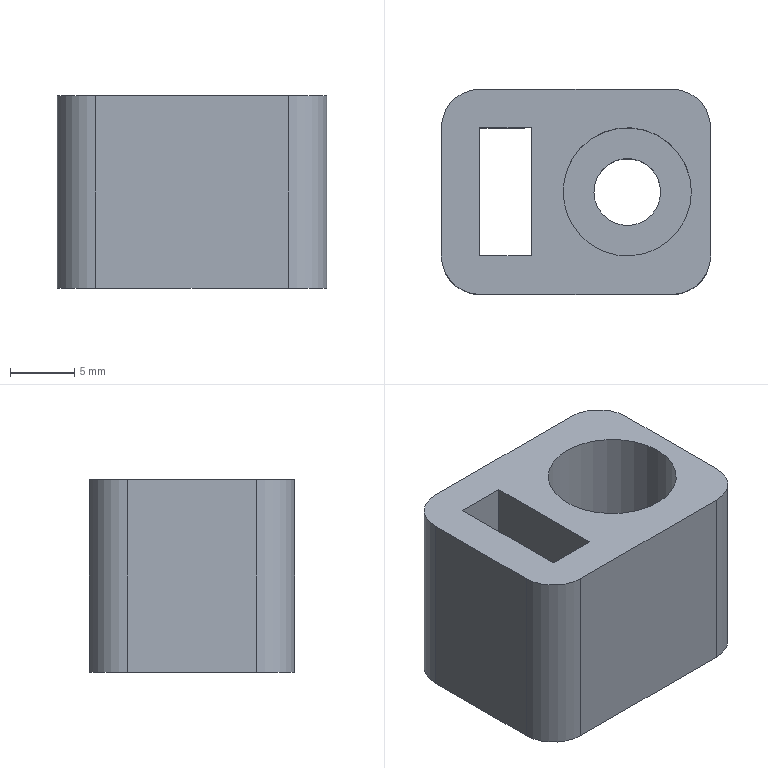Part | NX | features DIE-17 2 | 1 solid | 25 faces | box 21 x 16 x 15 mm | volume 3498 mm3 | plane 15 | cylinder 10 | commonest cylinder face diameters 2 x4 6 x4 5.206 x1 10 x1
STEP:
#1=CARTESIAN_POINT('',(2422.893,-834.621,858.716));
#2=VERTEX_POINT('',#1);
#3=CARTESIAN_POINT('',(2422.893,-834.621,846.716));
#4=VERTEX_POINT('',#3);
#5=CARTESIAN_POINT('',(2422.893,-834.621,858.516));
#6=DIRECTION('',(0.,0.,-1.));
#7=VECTOR('',#6,1000.);
#8=LINE('',#5,#7);
#9=EDGE_CURVE('',#2,#4,#8,.T.);
#10=ORIENTED_EDGE('',*,*,#9,.T.);
#11=CARTESIAN_POINT('',(2422.893,-844.621,846.716));
#12=VERTEX_POINT('',#11);
#13=CARTESIAN_POINT('',(2422.893,-833.746,846.716));
#14=DIRECTION('',(0.,1.,0.));
#15=VECTOR('',#14,1000.);
#16=LINE('',#13,#15);
#17=EDGE_CURVE('',#12,#4,#16,.T.);
#18=ORIENTED_EDGE('',*,*,#17,.F.);
#19=CARTESIAN_POINT('',(2422.893,-844.621,858.716));
#20=VERTEX_POINT('',#19);
#21=CARTESIAN_POINT('',(2422.893,-844.621,858.516));
#22=DIRECTION('',(0.,0.,-1.));
#23=VECTOR('',#22,1000.);
#24=LINE('',#21,#23);
#25=EDGE_CURVE('',#20,#12,#24,.T.);
#26=ORIENTED_EDGE('',*,*,#25,.F.);
#27=CARTESIAN_POINT('',(2422.893,-839.621,858.716));
#28=DIRECTION('',(0.,-1.,0.));
#29=VECTOR('',#28,1000.);
#30=LINE('',#27,#29);
#31=EDGE_CURVE('',#20,#2,#30,.F.);
#32=ORIENTED_EDGE('',*,*,#31,.T.);
#33=EDGE_LOOP('',(#10,#18,#26,#32));
#34=FACE_BOUND('',#33,.T.);
#35=CARTESIAN_POINT('',(2422.893,-837.246,858.516));
#36=DIRECTION('',(-1.,0.,0.));
#37=DIRECTION('',(0.,0.,1.));
#38=AXIS2_PLACEMENT_3D('',#35,#36,#37);
#39=PLANE('',#38);
#40=ADVANCED_FACE('',(#34),#39,.T.);
#41=CARTESIAN_POINT('',(2418.893,-834.621,858.716));
#42=VERTEX_POINT('',#41);
#43=CARTESIAN_POINT('',(2420.893,-834.621,858.716));
#44=DIRECTION('',(1.,0.,0.));
#45=VECTOR('',#44,1000.);
#46=LINE('',#43,#45);
#47=EDGE_CURVE('',#2,#42,#46,.F.);
#48=ORIENTED_EDGE('',*,*,#47,.F.);
#49=ORIENTED_EDGE('',*,*,#31,.F.);
#50=CARTESIAN_POINT('',(2418.893,-844.621,858.716));
#51=VERTEX_POINT('',#50);
#52=CARTESIAN_POINT('',(2420.893,-844.621,858.716));
#53=DIRECTION('',(1.,0.,0.));
#54=VECTOR('',#53,1000.);
#55=LINE('',#52,#54);
#56=EDGE_CURVE('',#20,#51,#55,.F.);
#57=ORIENTED_EDGE('',*,*,#56,.T.);
#58=CARTESIAN_POINT('',(2418.893,-837.871,858.716));
#59=DIRECTION('',(0.,-1.,0.));
#60=VECTOR('',#59,1000.);
#61=LINE('',#58,#60);
#62=EDGE_CURVE('',#42,#51,#61,.T.);
#63=ORIENTED_EDGE('',*,*,#62,.F.);
#64=EDGE_LOOP('',(#48,#49,#57,#63));
#65=FACE_BOUND('',#64,.T.);
#66=CARTESIAN_POINT('',(2415.893,-844.621,858.716));
#67=VERTEX_POINT('',#66);
#68=CARTESIAN_POINT('',(2418.893,-847.621,858.716));
#69=VERTEX_POINT('',#68);
#70=CARTESIAN_POINT('',(2418.893,-844.621,858.716));
#71=DIRECTION('',(0.,0.,1.));
#72=DIRECTION('',(1.,0.,0.));
#73=AXIS2_PLACEMENT_3D('',#70,#71,#72);
#74=CIRCLE('',#73,3.);
#75=EDGE_CURVE('',#67,#69,#74,.T.);
#76=ORIENTED_EDGE('',*,*,#75,.T.);
#77=CARTESIAN_POINT('',(2433.893,-847.621,858.716));
#78=VERTEX_POINT('',#77);
#79=CARTESIAN_POINT('',(2421.393,-847.621,858.716));
#80=DIRECTION('',(-1.,0.,0.));
#81=VECTOR('',#80,1000.);
#82=LINE('',#79,#81);
#83=EDGE_CURVE('',#78,#69,#82,.T.);
#84=ORIENTED_EDGE('',*,*,#83,.F.);
#85=CARTESIAN_POINT('',(2436.893,-844.621,858.716));
#86=VERTEX_POINT('',#85);
#87=CARTESIAN_POINT('',(2433.893,-844.621,858.716));
#88=DIRECTION('',(0.,0.,1.));
#89=DIRECTION('',(1.,0.,0.));
#90=AXIS2_PLACEMENT_3D('',#87,#88,#89);
#91=CIRCLE('',#90,3.);
#92=EDGE_CURVE('',#78,#86,#91,.T.);
#93=ORIENTED_EDGE('',*,*,#92,.T.);
#94=CARTESIAN_POINT('',(2436.893,-834.621,858.716));
#95=VERTEX_POINT('',#94);
#96=CARTESIAN_POINT('',(2436.893,-839.621,858.716));
#97=DIRECTION('',(0.,-1.,0.));
#98=VECTOR('',#97,1000.);
#99=LINE('',#96,#98);
#100=EDGE_CURVE('',#95,#86,#99,.T.);
#101=ORIENTED_EDGE('',*,*,#100,.F.);
#102=CARTESIAN_POINT('',(2433.893,-831.621,858.716));
#103=VERTEX_POINT('',#102);
#104=CARTESIAN_POINT('',(2433.893,-834.621,858.716));
#105=DIRECTION('',(0.,0.,1.));
#106=DIRECTION('',(1.,0.,0.));
#107=AXIS2_PLACEMENT_3D('',#104,#105,#106);
#108=CIRCLE('',#107,3.);
#109=EDGE_CURVE('',#95,#103,#108,.T.);
#110=ORIENTED_EDGE('',*,*,#109,.T.);
#111=CARTESIAN_POINT('',(2418.893,-831.621,858.716));
#112=VERTEX_POINT('',#111);
#113=CARTESIAN_POINT('',(2421.393,-831.621,858.716));
#114=DIRECTION('',(1.,0.,0.));
#115=VECTOR('',#114,1000.);
#116=LINE('',#113,#115);
#117=EDGE_CURVE('',#112,#103,#116,.T.);
#118=ORIENTED_EDGE('',*,*,#117,.F.);
#119=CARTESIAN_POINT('',(2415.893,-834.621,858.716));
#120=VERTEX_POINT('',#119);
#121=CARTESIAN_POINT('',(2418.893,-834.621,858.716));
#122=DIRECTION('',(0.,0.,1.));
#123=DIRECTION('',(1.,0.,0.));
#124=AXIS2_PLACEMENT_3D('',#121,#122,#123);
#125=CIRCLE('',#124,3.);
#126=EDGE_CURVE('',#112,#120,#125,.T.);
#127=ORIENTED_EDGE('',*,*,#126,.T.);
#128=CARTESIAN_POINT('',(2415.893,-839.621,858.716));
#129=DIRECTION('',(0.,1.,0.));
#130=VECTOR('',#129,1000.);
#131=LINE('',#128,#130);
#132=EDGE_CURVE('',#67,#120,#131,.T.);
#133=ORIENTED_EDGE('',*,*,#132,.F.);
#134=EDGE_LOOP('',(#76,#84,#93,#101,#110,#118,#127,#133));
#135=FACE_BOUND('',#134,.T.);
#136=CARTESIAN_POINT('',(2435.393,-839.621,858.716));
#137=VERTEX_POINT('',#136);
#138=CARTESIAN_POINT('',(2430.393,-839.621,858.716));
#139=DIRECTION('',(0.,0.,1.));
#140=DIRECTION('',(1.,0.,0.));
#141=AXIS2_PLACEMENT_3D('',#138,#139,#140);
#142=CIRCLE('',#141,5.);
#143=EDGE_CURVE('',#137,#137,#142,.T.);
#144=ORIENTED_EDGE('',*,*,#143,.F.);
#145=EDGE_LOOP('',(#144));
#146=FACE_BOUND('',#145,.T.);
#147=CARTESIAN_POINT('',(2421.393,-839.621,858.716));
#148=DIRECTION('',(0.,0.,1.));
#149=DIRECTION('',(1.,0.,0.));
#150=AXIS2_PLACEMENT_3D('',#147,#148,#149);
#151=PLANE('',#150);
#152=ADVANCED_FACE('',(#65,#135,#146),#151,.T.);
#153=CARTESIAN_POINT('',(2418.893,-844.621,843.716));
#154=VERTEX_POINT('',#153);
#155=CARTESIAN_POINT('',(2422.393,-844.621,843.716));
#156=VERTEX_POINT('',#155);
#157=CARTESIAN_POINT('',(2422.281,-844.621,843.716));
#158=DIRECTION('',(1.,0.,0.));
#159=VECTOR('',#158,1000.);
#160=LINE('',#157,#159);
#161=EDGE_CURVE('',#154,#156,#160,.T.);
#162=ORIENTED_EDGE('',*,*,#161,.T.);
#163=CARTESIAN_POINT('',(2423.259,-845.121,843.716));
#164=VERTEX_POINT('',#163);
#165=CARTESIAN_POINT('',(2423.259,-844.121,843.716));
#166=DIRECTION('',(0.,0.,-1.));
#167=DIRECTION('',(-1.,0.,0.));
#168=AXIS2_PLACEMENT_3D('',#165,#166,#167);
#169=CIRCLE('',#168,1.);
#170=EDGE_CURVE('',#156,#164,#169,.F.);
#171=ORIENTED_EDGE('',*,*,#170,.T.);
#172=CARTESIAN_POINT('',(2423.393,-845.121,843.716));
#173=VERTEX_POINT('',#172);
#174=CARTESIAN_POINT('',(2421.393,-845.121,843.716));
#175=DIRECTION('',(1.,0.,0.));
#176=VECTOR('',#175,1000.);
#177=LINE('',#174,#176);
#178=EDGE_CURVE('',#164,#173,#177,.T.);
#179=ORIENTED_EDGE('',*,*,#178,.T.);
#180=CARTESIAN_POINT('',(2424.393,-844.121,843.716));
#181=VERTEX_POINT('',#180);
#182=CARTESIAN_POINT('',(2423.393,-844.121,843.716));
#183=DIRECTION('',(0.,0.,-1.));
#184=DIRECTION('',(-1.,0.,0.));
#185=AXIS2_PLACEMENT_3D('',#182,#183,#184);
#186=CIRCLE('',#185,1.);
#187=EDGE_CURVE('',#173,#181,#186,.F.);
#188=ORIENTED_EDGE('',*,*,#187,.T.);
#189=CARTESIAN_POINT('',(2424.393,-835.121,843.716));
#190=VERTEX_POINT('',#189);
#191=CARTESIAN_POINT('',(2424.393,-833.746,843.716));
#192=DIRECTION('',(0.,-1.,0.));
#193=VECTOR('',#192,1000.);
#194=LINE('',#191,#193);
#195=EDGE_CURVE('',#190,#181,#194,.T.);
#196=ORIENTED_EDGE('',*,*,#195,.F.);
#197=CARTESIAN_POINT('',(2423.393,-834.121,843.716));
#198=VERTEX_POINT('',#197);
#199=CARTESIAN_POINT('',(2423.393,-835.121,843.716));
#200=DIRECTION('',(0.,0.,-1.));
#201=DIRECTION('',(-1.,0.,0.));
#202=AXIS2_PLACEMENT_3D('',#199,#200,#201);
#203=CIRCLE('',#202,1.);
#204=EDGE_CURVE('',#190,#198,#203,.F.);
#205=ORIENTED_EDGE('',*,*,#204,.T.);
#206=CARTESIAN_POINT('',(2423.259,-834.121,843.716));
#207=VERTEX_POINT('',#206);
#208=CARTESIAN_POINT('',(2421.393,-834.121,843.716));
#209=DIRECTION('',(-1.,0.,0.));
#210=VECTOR('',#209,1000.);
#211=LINE('',#208,#210);
#212=EDGE_CURVE('',#198,#207,#211,.T.);
#213=ORIENTED_EDGE('',*,*,#212,.T.);
#214=CARTESIAN_POINT('',(2422.393,-834.621,843.716));
#215=VERTEX_POINT('',#214);
#216=CARTESIAN_POINT('',(2423.259,-835.121,843.716));
#217=DIRECTION('',(0.,0.,-1.));
#218=DIRECTION('',(-1.,0.,0.));
#219=AXIS2_PLACEMENT_3D('',#216,#217,#218);
#220=CIRCLE('',#219,1.);
#221=EDGE_CURVE('',#207,#215,#220,.F.);
#222=ORIENTED_EDGE('',*,*,#221,.T.);
#223=CARTESIAN_POINT('',(2418.893,-834.621,843.716));
#224=VERTEX_POINT('',#223);
#225=CARTESIAN_POINT('',(2422.281,-834.621,843.716));
#226=DIRECTION('',(-1.,0.,0.));
#227=VECTOR('',#226,1000.);
#228=LINE('',#225,#227);
#229=EDGE_CURVE('',#215,#224,#228,.T.);
#230=ORIENTED_EDGE('',*,*,#229,.T.);
#231=CARTESIAN_POINT('',(2418.893,-833.746,843.716));
#232=DIRECTION('',(0.,-1.,0.));
#233=VECTOR('',#232,1000.);
#234=LINE('',#231,#233);
#235=EDGE_CURVE('',#224,#154,#234,.T.);
#236=ORIENTED_EDGE('',*,*,#235,.T.);
#237=EDGE_LOOP('',(#162,#171,#179,#188,#196,#205,#213,#222,#230,#236));
#238=FACE_BOUND('',#237,.T.);
#239=CARTESIAN_POINT('',(2427.79,-839.621,843.716));
#240=VERTEX_POINT('',#239);
#241=CARTESIAN_POINT('',(2430.393,-839.621,843.716));
#242=DIRECTION('',(0.,0.,-1.));
#243=DIRECTION('',(-1.,0.,0.));
#244=AXIS2_PLACEMENT_3D('',#241,#242,#243);
#245=CIRCLE('',#244,2.603);
#246=EDGE_CURVE('',#240,#240,#245,.T.);
#247=ORIENTED_EDGE('',*,*,#246,.F.);
#248=EDGE_LOOP('',(#247));
#249=FACE_BOUND('',#248,.T.);
#250=CARTESIAN_POINT('',(2418.893,-847.621,843.716));
#251=VERTEX_POINT('',#250);
#252=CARTESIAN_POINT('',(2433.893,-847.621,843.716));
#253=VERTEX_POINT('',#252);
#254=CARTESIAN_POINT('',(2421.393,-847.621,843.716));
#255=DIRECTION('',(1.,0.,0.));
#256=VECTOR('',#255,1000.);
#257=LINE('',#254,#256);
#258=EDGE_CURVE('',#251,#253,#257,.T.);
#259=ORIENTED_EDGE('',*,*,#258,.F.);
#260=CARTESIAN_POINT('',(2415.893,-844.621,843.716));
#261=VERTEX_POINT('',#260);
#262=CARTESIAN_POINT('',(2418.893,-844.621,843.716));
#263=DIRECTION('',(0.,0.,-1.));
#264=DIRECTION('',(-1.,0.,0.));
#265=AXIS2_PLACEMENT_3D('',#262,#263,#264);
#266=CIRCLE('',#265,3.);
#267=EDGE_CURVE('',#251,#261,#266,.T.);
#268=ORIENTED_EDGE('',*,*,#267,.T.);
#269=CARTESIAN_POINT('',(2415.893,-834.621,843.716));
#270=VERTEX_POINT('',#269);
#271=CARTESIAN_POINT('',(2415.893,-839.621,843.716));
#272=DIRECTION('',(0.,-1.,0.));
#273=VECTOR('',#272,1000.);
#274=LINE('',#271,#273);
#275=EDGE_CURVE('',#270,#261,#274,.T.);
#276=ORIENTED_EDGE('',*,*,#275,.F.);
#277=CARTESIAN_POINT('',(2418.893,-831.621,843.716));
#278=VERTEX_POINT('',#277);
#279=CARTESIAN_POINT('',(2418.893,-834.621,843.716));
#280=DIRECTION('',(0.,0.,-1.));
#281=DIRECTION('',(-1.,0.,0.));
#282=AXIS2_PLACEMENT_3D('',#279,#280,#281);
#283=CIRCLE('',#282,3.);
#284=EDGE_CURVE('',#270,#278,#283,.T.);
#285=ORIENTED_EDGE('',*,*,#284,.T.);
#286=CARTESIAN_POINT('',(2433.893,-831.621,843.716));
#287=VERTEX_POINT('',#286);
#288=CARTESIAN_POINT('',(2421.393,-831.621,843.716));
#289=DIRECTION('',(-1.,0.,0.));
#290=VECTOR('',#289,1000.);
#291=LINE('',#288,#290);
#292=EDGE_CURVE('',#287,#278,#291,.T.);
#293=ORIENTED_EDGE('',*,*,#292,.F.);
#294=CARTESIAN_POINT('',(2436.893,-834.621,843.716));
#295=VERTEX_POINT('',#294);
#296=CARTESIAN_POINT('',(2433.893,-834.621,843.716));
#297=DIRECTION('',(0.,0.,-1.));
#298=DIRECTION('',(-1.,0.,0.));
#299=AXIS2_PLACEMENT_3D('',#296,#297,#298);
#300=CIRCLE('',#299,3.);
#301=EDGE_CURVE('',#287,#295,#300,.T.);
#302=ORIENTED_EDGE('',*,*,#301,.T.);
#303=CARTESIAN_POINT('',(2436.893,-844.621,843.716));
#304=VERTEX_POINT('',#303);
#305=CARTESIAN_POINT('',(2436.893,-839.621,843.716));
#306=DIRECTION('',(0.,1.,0.));
#307=VECTOR('',#306,1000.);
#308=LINE('',#305,#307);
#309=EDGE_CURVE('',#304,#295,#308,.T.);
#310=ORIENTED_EDGE('',*,*,#309,.F.);
#311=CARTESIAN_POINT('',(2433.893,-844.621,843.716));
#312=DIRECTION('',(0.,0.,-1.));
#313=DIRECTION('',(-1.,0.,0.));
#314=AXIS2_PLACEMENT_3D('',#311,#312,#313);
#315=CIRCLE('',#314,3.);
#316=EDGE_CURVE('',#304,#253,#315,.T.);
#317=ORIENTED_EDGE('',*,*,#316,.T.);
#318=EDGE_LOOP('',(#259,#268,#276,#285,#293,#302,#310,#317));
#319=FACE_BOUND('',#318,.T.);
#320=CARTESIAN_POINT('',(2421.393,-839.621,843.716));
#321=DIRECTION('',(0.,0.,-1.));
#322=DIRECTION('',(-1.,0.,0.));
#323=AXIS2_PLACEMENT_3D('',#320,#321,#322);
#324=PLANE('',#323);
#325=ADVANCED_FACE('',(#238,#249,#319),#324,.T.);
#326=ORIENTED_EDGE('',*,*,#83,.T.);
#327=CARTESIAN_POINT('',(2418.893,-847.621,840.716));
#328=DIRECTION('',(0.,0.,1.));
#329=VECTOR('',#328,1000.);
#330=LINE('',#327,#329);
#331=EDGE_CURVE('',#69,#251,#330,.F.);
#332=ORIENTED_EDGE('',*,*,#331,.T.);
#333=ORIENTED_EDGE('',*,*,#258,.T.);
#334=CARTESIAN_POINT('',(2433.893,-847.621,840.716));
#335=DIRECTION('',(0.,0.,1.));
#336=VECTOR('',#335,1000.);
#337=LINE('',#334,#336);
#338=EDGE_CURVE('',#253,#78,#337,.T.);
#339=ORIENTED_EDGE('',*,*,#338,.T.);
#340=EDGE_LOOP('',(#326,#332,#333,#339));
#341=FACE_BOUND('',#340,.T.);
#342=CARTESIAN_POINT('',(2421.393,-847.621,840.716));
#343=DIRECTION('',(0.,-1.,0.));
#344=DIRECTION('',(0.,0.,-1.));
#345=AXIS2_PLACEMENT_3D('',#342,#343,#344);
#346=PLANE('',#345);
#347=ADVANCED_FACE('',(#341),#346,.T.);
#348=ORIENTED_EDGE('',*,*,#292,.T.);
#349=CARTESIAN_POINT('',(2418.893,-831.621,840.716));
#350=DIRECTION('',(0.,0.,1.));
#351=VECTOR('',#350,1000.);
#352=LINE('',#349,#351);
#353=EDGE_CURVE('',#278,#112,#352,.T.);
#354=ORIENTED_EDGE('',*,*,#353,.T.);
#355=ORIENTED_EDGE('',*,*,#117,.T.);
#356=CARTESIAN_POINT('',(2433.893,-831.621,840.716));
#357=DIRECTION('',(0.,0.,1.));
#358=VECTOR('',#357,1000.);
#359=LINE('',#356,#358);
#360=EDGE_CURVE('',#103,#287,#359,.F.);
#361=ORIENTED_EDGE('',*,*,#360,.T.);
#362=EDGE_LOOP('',(#348,#354,#355,#361));
#363=FACE_BOUND('',#362,.T.);
#364=CARTESIAN_POINT('',(2421.393,-831.621,840.716));
#365=DIRECTION('',(0.,1.,0.));
#366=DIRECTION('',(0.,0.,1.));
#367=AXIS2_PLACEMENT_3D('',#364,#365,#366);
#368=PLANE('',#367);
#369=ADVANCED_FACE('',(#363),#368,.T.);
#370=ORIENTED_EDGE('',*,*,#212,.F.);
#371=CARTESIAN_POINT('',(2423.393,-834.121,846.716));
#372=VERTEX_POINT('',#371);
#373=CARTESIAN_POINT('',(2423.393,-834.121,846.716));
#374=DIRECTION('',(0.,0.,-1.));
#375=VECTOR('',#374,1000.);
#376=LINE('',#373,#375);
#377=EDGE_CURVE('',#198,#372,#376,.F.);
#378=ORIENTED_EDGE('',*,*,#377,.T.);
#379=CARTESIAN_POINT('',(2423.259,-834.121,846.716));
#380=VERTEX_POINT('',#379);
#381=CARTESIAN_POINT('',(2423.393,-834.121,846.716));
#382=DIRECTION('',(1.,0.,0.));
#383=VECTOR('',#382,1000.);
#384=LINE('',#381,#383);
#385=EDGE_CURVE('',#380,#372,#384,.T.);
#386=ORIENTED_EDGE('',*,*,#385,.F.);
#387=CARTESIAN_POINT('',(2423.259,-834.121,843.716));
#388=DIRECTION('',(0.,0.,-1.));
#389=VECTOR('',#388,1000.);
#390=LINE('',#387,#389);
#391=EDGE_CURVE('',#380,#207,#390,.T.);
#392=ORIENTED_EDGE('',*,*,#391,.T.);
#393=EDGE_LOOP('',(#370,#378,#386,#392));
#394=FACE_BOUND('',#393,.T.);
#395=CARTESIAN_POINT('',(2422.281,-834.121,858.516));
#396=DIRECTION('',(0.,-1.,0.));
#397=DIRECTION('',(0.,0.,-1.));
#398=AXIS2_PLACEMENT_3D('',#395,#396,#397);
#399=PLANE('',#398);
#400=ADVANCED_FACE('',(#394),#399,.T.);
#401=ORIENTED_EDGE('',*,*,#178,.F.);
#402=CARTESIAN_POINT('',(2423.259,-845.121,846.716));
#403=VERTEX_POINT('',#402);
#404=CARTESIAN_POINT('',(2423.259,-845.121,846.716));
#405=DIRECTION('',(0.,0.,1.));
#406=VECTOR('',#405,1000.);
#407=LINE('',#404,#406);
#408=EDGE_CURVE('',#164,#403,#407,.T.);
#409=ORIENTED_EDGE('',*,*,#408,.T.);
#410=CARTESIAN_POINT('',(2423.393,-845.121,846.716));
#411=VERTEX_POINT('',#410);
#412=CARTESIAN_POINT('',(2422.281,-845.121,846.716));
#413=DIRECTION('',(1.,0.,0.));
#414=VECTOR('',#413,1000.);
#415=LINE('',#412,#414);
#416=EDGE_CURVE('',#403,#411,#415,.T.);
#417=ORIENTED_EDGE('',*,*,#416,.T.);
#418=CARTESIAN_POINT('',(2423.393,-845.121,843.716));
#419=DIRECTION('',(0.,0.,-1.));
#420=VECTOR('',#419,1000.);
#421=LINE('',#418,#420);
#422=EDGE_CURVE('',#411,#173,#421,.T.);
#423=ORIENTED_EDGE('',*,*,#422,.T.);
#424=EDGE_LOOP('',(#401,#409,#417,#423));
#425=FACE_BOUND('',#424,.T.);
#426=CARTESIAN_POINT('',(2422.281,-845.121,858.516));
#427=DIRECTION('',(0.,1.,0.));
#428=DIRECTION('',(0.,0.,-1.));
#429=AXIS2_PLACEMENT_3D('',#426,#427,#428);
#430=PLANE('',#429);
#431=ADVANCED_FACE('',(#425),#430,.T.);
#432=ORIENTED_EDGE('',*,*,#309,.T.);
#433=CARTESIAN_POINT('',(2436.893,-834.621,840.716));
#434=DIRECTION('',(0.,0.,1.));
#435=VECTOR('',#434,1000.);
#436=LINE('',#433,#435);
#437=EDGE_CURVE('',#295,#95,#436,.T.);
#438=ORIENTED_EDGE('',*,*,#437,.T.);
#439=ORIENTED_EDGE('',*,*,#100,.T.);
#440=CARTESIAN_POINT('',(2436.893,-844.621,840.716));
#441=DIRECTION('',(0.,0.,1.));
#442=VECTOR('',#441,1000.);
#443=LINE('',#440,#442);
#444=EDGE_CURVE('',#86,#304,#443,.F.);
#445=ORIENTED_EDGE('',*,*,#444,.T.);
#446=EDGE_LOOP('',(#432,#438,#439,#445));
#447=FACE_BOUND('',#446,.T.);
#448=CARTESIAN_POINT('',(2436.893,-839.621,840.716));
#449=DIRECTION('',(1.,0.,0.));
#450=DIRECTION('',(0.,0.,-1.));
#451=AXIS2_PLACEMENT_3D('',#448,#449,#450);
#452=PLANE('',#451);
#453=ADVANCED_FACE('',(#447),#452,.T.);
#454=ORIENTED_EDGE('',*,*,#301,.F.);
#455=ORIENTED_EDGE('',*,*,#360,.F.);
#456=ORIENTED_EDGE('',*,*,#109,.F.);
#457=ORIENTED_EDGE('',*,*,#437,.F.);
#458=EDGE_LOOP('',(#454,#455,#456,#457));
#459=FACE_BOUND('',#458,.T.);
#460=CARTESIAN_POINT('',(2433.893,-834.621,840.716));
#461=DIRECTION('',(0.,0.,1.));
#462=DIRECTION('',(1.,0.,0.));
#463=AXIS2_PLACEMENT_3D('',#460,#461,#462);
#464=CYLINDRICAL_SURFACE('',#463,3.);
#465=ADVANCED_FACE('',(#459),#464,.T.);
#466=ORIENTED_EDGE('',*,*,#316,.F.);
#467=ORIENTED_EDGE('',*,*,#444,.F.);
#468=ORIENTED_EDGE('',*,*,#92,.F.);
#469=ORIENTED_EDGE('',*,*,#338,.F.);
#470=EDGE_LOOP('',(#466,#467,#468,#469));
#471=FACE_BOUND('',#470,.T.);
#472=CARTESIAN_POINT('',(2433.893,-844.621,840.716));
#473=DIRECTION('',(0.,0.,1.));
#474=DIRECTION('',(1.,0.,0.));
#475=AXIS2_PLACEMENT_3D('',#472,#473,#474);
#476=CYLINDRICAL_SURFACE('',#475,3.);
#477=ADVANCED_FACE('',(#471),#476,.T.);
#478=ORIENTED_EDGE('',*,*,#246,.T.);
#479=EDGE_LOOP('',(#478));
#480=FACE_BOUND('',#479,.T.);
#481=CARTESIAN_POINT('',(2432.996,-839.621,850.716));
#482=VERTEX_POINT('',#481);
#483=CARTESIAN_POINT('',(2430.393,-839.621,850.716));
#484=DIRECTION('',(0.,0.,1.));
#485=DIRECTION('',(1.,0.,0.));
#486=AXIS2_PLACEMENT_3D('',#483,#484,#485);
#487=CIRCLE('',#486,2.603);
#488=EDGE_CURVE('',#482,#482,#487,.T.);
#489=ORIENTED_EDGE('',*,*,#488,.T.);
#490=EDGE_LOOP('',(#489));
#491=FACE_BOUND('',#490,.T.);
#492=CARTESIAN_POINT('',(2430.393,-839.621,842.716));
#493=DIRECTION('',(0.,0.,1.));
#494=DIRECTION('',(1.,0.,0.));
#495=AXIS2_PLACEMENT_3D('',#492,#493,#494);
#496=CYLINDRICAL_SURFACE('',#495,2.603);
#497=ADVANCED_FACE('',(#480,#491),#496,.F.);
#498=ORIENTED_EDGE('',*,*,#143,.T.);
#499=EDGE_LOOP('',(#498));
#500=FACE_BOUND('',#499,.T.);
#501=CARTESIAN_POINT('',(2435.393,-839.621,850.716));
#502=VERTEX_POINT('',#501);
#503=CARTESIAN_POINT('',(2430.393,-839.621,850.716));
#504=DIRECTION('',(0.,0.,1.));
#505=DIRECTION('',(1.,0.,0.));
#506=AXIS2_PLACEMENT_3D('',#503,#504,#505);
#507=CIRCLE('',#506,5.);
#508=EDGE_CURVE('',#502,#502,#507,.F.);
#509=ORIENTED_EDGE('',*,*,#508,.T.);
#510=EDGE_LOOP('',(#509));
#511=FACE_BOUND('',#510,.T.);
#512=CARTESIAN_POINT('',(2430.393,-839.621,850.716));
#513=DIRECTION('',(0.,0.,1.));
#514=DIRECTION('',(1.,0.,0.));
#515=AXIS2_PLACEMENT_3D('',#512,#513,#514);
#516=CYLINDRICAL_SURFACE('',#515,5.);
#517=ADVANCED_FACE('',(#500,#511),#516,.F.);
#518=ORIENTED_EDGE('',*,*,#488,.F.);
#519=EDGE_LOOP('',(#518));
#520=FACE_BOUND('',#519,.T.);
#521=ORIENTED_EDGE('',*,*,#508,.F.);
#522=EDGE_LOOP('',(#521));
#523=FACE_BOUND('',#522,.T.);
#524=CARTESIAN_POINT('',(2430.393,-839.621,850.716));
#525=DIRECTION('',(0.,0.,1.));
#526=DIRECTION('',(1.,0.,0.));
#527=AXIS2_PLACEMENT_3D('',#524,#525,#526);
#528=PLANE('',#527);
#529=ADVANCED_FACE('',(#520,#523),#528,.T.);
#530=ORIENTED_EDGE('',*,*,#385,.T.);
#531=CARTESIAN_POINT('',(2424.393,-835.121,846.716));
#532=VERTEX_POINT('',#531);
#533=CARTESIAN_POINT('',(2423.393,-835.121,846.716));
#534=DIRECTION('',(0.,0.,1.));
#535=DIRECTION('',(1.,0.,0.));
#536=AXIS2_PLACEMENT_3D('',#533,#534,#535);
#537=CIRCLE('',#536,1.);
#538=EDGE_CURVE('',#372,#532,#537,.F.);
#539=ORIENTED_EDGE('',*,*,#538,.T.);
#540=CARTESIAN_POINT('',(2424.393,-844.121,846.716));
#541=VERTEX_POINT('',#540);
#542=CARTESIAN_POINT('',(2424.393,-834.371,846.716));
#543=DIRECTION('',(0.,-1.,0.));
#544=VECTOR('',#543,1000.);
#545=LINE('',#542,#544);
#546=EDGE_CURVE('',#532,#541,#545,.T.);
#547=ORIENTED_EDGE('',*,*,#546,.T.);
#548=CARTESIAN_POINT('',(2423.393,-844.121,846.716));
#549=DIRECTION('',(0.,0.,1.));
#550=DIRECTION('',(1.,0.,0.));
#551=AXIS2_PLACEMENT_3D('',#548,#549,#550);
#552=CIRCLE('',#551,1.);
#553=EDGE_CURVE('',#541,#411,#552,.F.);
#554=ORIENTED_EDGE('',*,*,#553,.T.);
#555=ORIENTED_EDGE('',*,*,#416,.F.);
#556=CARTESIAN_POINT('',(2422.393,-844.621,846.716));
#557=VERTEX_POINT('',#556);
#558=CARTESIAN_POINT('',(2423.259,-844.121,846.716));
#559=DIRECTION('',(0.,0.,1.));
#560=DIRECTION('',(1.,0.,0.));
#561=AXIS2_PLACEMENT_3D('',#558,#559,#560);
#562=CIRCLE('',#561,1.);
#563=EDGE_CURVE('',#403,#557,#562,.F.);
#564=ORIENTED_EDGE('',*,*,#563,.T.);
#565=CARTESIAN_POINT('',(2423.393,-844.621,846.716));
#566=DIRECTION('',(-1.,0.,0.));
#567=VECTOR('',#566,1000.);
#568=LINE('',#565,#567);
#569=EDGE_CURVE('',#12,#557,#568,.T.);
#570=ORIENTED_EDGE('',*,*,#569,.F.);
#571=ORIENTED_EDGE('',*,*,#17,.T.);
#572=CARTESIAN_POINT('',(2422.393,-834.621,846.716));
#573=VERTEX_POINT('',#572);
#574=CARTESIAN_POINT('',(2422.281,-834.621,846.716));
#575=DIRECTION('',(-1.,0.,0.));
#576=VECTOR('',#575,1000.);
#577=LINE('',#574,#576);
#578=EDGE_CURVE('',#4,#573,#577,.T.);
#579=ORIENTED_EDGE('',*,*,#578,.T.);
#580=CARTESIAN_POINT('',(2423.259,-835.121,846.716));
#581=DIRECTION('',(0.,0.,1.));
#582=DIRECTION('',(1.,0.,0.));
#583=AXIS2_PLACEMENT_3D('',#580,#581,#582);
#584=CIRCLE('',#583,1.);
#585=EDGE_CURVE('',#573,#380,#584,.F.);
#586=ORIENTED_EDGE('',*,*,#585,.T.);
#587=EDGE_LOOP('',(#530,#539,#547,#554,#555,#564,#570,#571,#579,#586));
#588=FACE_BOUND('',#587,.T.);
#589=CARTESIAN_POINT('',(2423.393,-834.371,846.716));
#590=DIRECTION('',(0.,0.,1.));
#591=DIRECTION('',(1.,0.,0.));
#592=AXIS2_PLACEMENT_3D('',#589,#590,#591);
#593=PLANE('',#592);
#594=ADVANCED_FACE('',(#588),#593,.F.);
#595=ORIENTED_EDGE('',*,*,#546,.F.);
#596=CARTESIAN_POINT('',(2424.393,-835.121,843.716));
#597=DIRECTION('',(0.,0.,-1.));
#598=VECTOR('',#597,1000.);
#599=LINE('',#596,#598);
#600=EDGE_CURVE('',#532,#190,#599,.T.);
#601=ORIENTED_EDGE('',*,*,#600,.T.);
#602=ORIENTED_EDGE('',*,*,#195,.T.);
#603=CARTESIAN_POINT('',(2424.393,-844.121,846.716));
#604=DIRECTION('',(0.,0.,-1.));
#605=VECTOR('',#604,1000.);
#606=LINE('',#603,#605);
#607=EDGE_CURVE('',#181,#541,#606,.F.);
#608=ORIENTED_EDGE('',*,*,#607,.T.);
#609=EDGE_LOOP('',(#595,#601,#602,#608));
#610=FACE_BOUND('',#609,.T.);
#611=CARTESIAN_POINT('',(2424.393,-833.746,858.516));
#612=DIRECTION('',(-1.,0.,0.));
#613=DIRECTION('',(0.,0.,1.));
#614=AXIS2_PLACEMENT_3D('',#611,#612,#613);
#615=PLANE('',#614);
#616=ADVANCED_FACE('',(#610),#615,.T.);
#617=ORIENTED_EDGE('',*,*,#132,.T.);
#618=CARTESIAN_POINT('',(2415.893,-834.621,840.716));
#619=DIRECTION('',(0.,0.,1.));
#620=VECTOR('',#619,1000.);
#621=LINE('',#618,#620);
#622=EDGE_CURVE('',#120,#270,#621,.F.);
#623=ORIENTED_EDGE('',*,*,#622,.T.);
#624=ORIENTED_EDGE('',*,*,#275,.T.);
#625=CARTESIAN_POINT('',(2415.893,-844.621,840.716));
#626=DIRECTION('',(0.,0.,1.));
#627=VECTOR('',#626,1000.);
#628=LINE('',#625,#627);
#629=EDGE_CURVE('',#261,#67,#628,.T.);
#630=ORIENTED_EDGE('',*,*,#629,.T.);
#631=EDGE_LOOP('',(#617,#623,#624,#630));
#632=FACE_BOUND('',#631,.T.);
#633=CARTESIAN_POINT('',(2415.893,-839.621,840.716));
#634=DIRECTION('',(-1.,0.,0.));
#635=DIRECTION('',(0.,0.,1.));
#636=AXIS2_PLACEMENT_3D('',#633,#634,#635);
#637=PLANE('',#636);
#638=ADVANCED_FACE('',(#632),#637,.T.);
#639=ORIENTED_EDGE('',*,*,#267,.F.);
#640=ORIENTED_EDGE('',*,*,#331,.F.);
#641=ORIENTED_EDGE('',*,*,#75,.F.);
#642=ORIENTED_EDGE('',*,*,#629,.F.);
#643=EDGE_LOOP('',(#639,#640,#641,#642));
#644=FACE_BOUND('',#643,.T.);
#645=CARTESIAN_POINT('',(2418.893,-844.621,840.716));
#646=DIRECTION('',(0.,0.,1.));
#647=DIRECTION('',(1.,0.,0.));
#648=AXIS2_PLACEMENT_3D('',#645,#646,#647);
#649=CYLINDRICAL_SURFACE('',#648,3.);
#650=ADVANCED_FACE('',(#644),#649,.T.);
#651=ORIENTED_EDGE('',*,*,#284,.F.);
#652=ORIENTED_EDGE('',*,*,#622,.F.);
#653=ORIENTED_EDGE('',*,*,#126,.F.);
#654=ORIENTED_EDGE('',*,*,#353,.F.);
#655=EDGE_LOOP('',(#651,#652,#653,#654));
#656=FACE_BOUND('',#655,.T.);
#657=CARTESIAN_POINT('',(2418.893,-834.621,840.716));
#658=DIRECTION('',(0.,0.,1.));
#659=DIRECTION('',(1.,0.,0.));
#660=AXIS2_PLACEMENT_3D('',#657,#658,#659);
#661=CYLINDRICAL_SURFACE('',#660,3.);
#662=ADVANCED_FACE('',(#656),#661,.T.);
#663=ORIENTED_EDGE('',*,*,#62,.T.);
#664=CARTESIAN_POINT('',(2418.893,-844.621,858.516));
#665=DIRECTION('',(0.,0.,-1.));
#666=VECTOR('',#665,1000.);
#667=LINE('',#664,#666);
#668=EDGE_CURVE('',#51,#154,#667,.T.);
#669=ORIENTED_EDGE('',*,*,#668,.T.);
#670=ORIENTED_EDGE('',*,*,#235,.F.);
#671=CARTESIAN_POINT('',(2418.893,-834.621,858.516));
#672=DIRECTION('',(0.,0.,-1.));
#673=VECTOR('',#672,1000.);
#674=LINE('',#671,#673);
#675=EDGE_CURVE('',#42,#224,#674,.T.);
#676=ORIENTED_EDGE('',*,*,#675,.F.);
#677=EDGE_LOOP('',(#663,#669,#670,#676));
#678=FACE_BOUND('',#677,.T.);
#679=CARTESIAN_POINT('',(2418.893,-837.246,858.516));
#680=DIRECTION('',(1.,0.,0.));
#681=DIRECTION('',(0.,0.,1.));
#682=AXIS2_PLACEMENT_3D('',#679,#680,#681);
#683=PLANE('',#682);
#684=ADVANCED_FACE('',(#678),#683,.T.);
#685=ORIENTED_EDGE('',*,*,#25,.T.);
#686=ORIENTED_EDGE('',*,*,#569,.T.);
#687=CARTESIAN_POINT('',(2422.393,-844.621,852.716));
#688=DIRECTION('',(0.,0.,-1.));
#689=VECTOR('',#688,1000.);
#690=LINE('',#687,#689);
#691=EDGE_CURVE('',#557,#156,#690,.T.);
#692=ORIENTED_EDGE('',*,*,#691,.T.);
#693=ORIENTED_EDGE('',*,*,#161,.F.);
#694=ORIENTED_EDGE('',*,*,#668,.F.);
#695=ORIENTED_EDGE('',*,*,#56,.F.);
#696=EDGE_LOOP('',(#685,#686,#692,#693,#694,#695));
#697=FACE_BOUND('',#696,.T.);
#698=CARTESIAN_POINT('',(2422.281,-844.621,858.516));
#699=DIRECTION('',(0.,1.,0.));
#700=DIRECTION('',(0.,0.,-1.));
#701=AXIS2_PLACEMENT_3D('',#698,#699,#700);
#702=PLANE('',#701);
#703=ADVANCED_FACE('',(#697),#702,.T.);
#704=ORIENTED_EDGE('',*,*,#229,.F.);
#705=CARTESIAN_POINT('',(2422.393,-834.621,858.516));
#706=DIRECTION('',(0.,0.,-1.));
#707=VECTOR('',#706,1000.);
#708=LINE('',#705,#707);
#709=EDGE_CURVE('',#573,#215,#708,.T.);
#710=ORIENTED_EDGE('',*,*,#709,.F.);
#711=ORIENTED_EDGE('',*,*,#578,.F.);
#712=ORIENTED_EDGE('',*,*,#9,.F.);
#713=ORIENTED_EDGE('',*,*,#47,.T.);
#714=ORIENTED_EDGE('',*,*,#675,.T.);
#715=EDGE_LOOP('',(#704,#710,#711,#712,#713,#714));
#716=FACE_BOUND('',#715,.T.);
#717=CARTESIAN_POINT('',(2422.281,-834.621,858.516));
#718=DIRECTION('',(0.,-1.,0.));
#719=DIRECTION('',(0.,0.,-1.));
#720=AXIS2_PLACEMENT_3D('',#717,#718,#719);
#721=PLANE('',#720);
#722=ADVANCED_FACE('',(#716),#721,.T.);
#723=ORIENTED_EDGE('',*,*,#538,.F.);
#724=ORIENTED_EDGE('',*,*,#377,.F.);
#725=ORIENTED_EDGE('',*,*,#204,.F.);
#726=ORIENTED_EDGE('',*,*,#600,.F.);
#727=EDGE_LOOP('',(#723,#724,#725,#726));
#728=FACE_BOUND('',#727,.T.);
#729=CARTESIAN_POINT('',(2423.393,-835.121,858.516));
#730=DIRECTION('',(0.,0.,1.));
#731=DIRECTION('',(1.,0.,0.));
#732=AXIS2_PLACEMENT_3D('',#729,#730,#731);
#733=CYLINDRICAL_SURFACE('',#732,1.);
#734=ADVANCED_FACE('',(#728),#733,.F.);
#735=ORIENTED_EDGE('',*,*,#585,.F.);
#736=ORIENTED_EDGE('',*,*,#709,.T.);
#737=ORIENTED_EDGE('',*,*,#221,.F.);
#738=ORIENTED_EDGE('',*,*,#391,.F.);
#739=EDGE_LOOP('',(#735,#736,#737,#738));
#740=FACE_BOUND('',#739,.T.);
#741=CARTESIAN_POINT('',(2423.259,-835.121,852.716));
#742=DIRECTION('',(0.,0.,1.));
#743=DIRECTION('',(1.,0.,0.));
#744=AXIS2_PLACEMENT_3D('',#741,#742,#743);
#745=CYLINDRICAL_SURFACE('',#744,1.);
#746=ADVANCED_FACE('',(#740),#745,.F.);
#747=ORIENTED_EDGE('',*,*,#170,.F.);
#748=ORIENTED_EDGE('',*,*,#691,.F.);
#749=ORIENTED_EDGE('',*,*,#563,.F.);
#750=ORIENTED_EDGE('',*,*,#408,.F.);
#751=EDGE_LOOP('',(#747,#748,#749,#750));
#752=FACE_BOUND('',#751,.T.);
#753=CARTESIAN_POINT('',(2423.259,-844.121,852.716));
#754=DIRECTION('',(0.,0.,-1.));
#755=DIRECTION('',(-1.,0.,0.));
#756=AXIS2_PLACEMENT_3D('',#753,#754,#755);
#757=CYLINDRICAL_SURFACE('',#756,1.);
#758=ADVANCED_FACE('',(#752),#757,.F.);
#759=ORIENTED_EDGE('',*,*,#553,.F.);
#760=ORIENTED_EDGE('',*,*,#607,.F.);
#761=ORIENTED_EDGE('',*,*,#187,.F.);
#762=ORIENTED_EDGE('',*,*,#422,.F.);
#763=EDGE_LOOP('',(#759,#760,#761,#762));
#764=FACE_BOUND('',#763,.T.);
#765=CARTESIAN_POINT('',(2423.393,-844.121,858.516));
#766=DIRECTION('',(0.,0.,1.));
#767=DIRECTION('',(1.,0.,0.));
#768=AXIS2_PLACEMENT_3D('',#765,#766,#767);
#769=CYLINDRICAL_SURFACE('',#768,1.);
#770=ADVANCED_FACE('',(#764),#769,.F.);
#771=CLOSED_SHELL('',(#40,#152,#325,#347,#369,#400,#431,#453,#465,#477,#497,#517,#529,#594,#616,#638,#650,#662,#684,#703,#722,#734,#746,#758,#770));
#772=MANIFOLD_SOLID_BREP('',#771);
#773=(LENGTH_UNIT()NAMED_UNIT(*)SI_UNIT(.MILLI.,.METRE.));
#774=UNCERTAINTY_MEASURE_WITH_UNIT(LENGTH_MEASURE(0.00001),#773,'','');
#775=(NAMED_UNIT(*)PLANE_ANGLE_UNIT()SI_UNIT($,.RADIAN.));
#776=(NAMED_UNIT(*)SI_UNIT($,.STERADIAN.)SOLID_ANGLE_UNIT());
#777=(GEOMETRIC_REPRESENTATION_CONTEXT(3)GLOBAL_UNCERTAINTY_ASSIGNED_CONTEXT((#774))GLOBAL_UNIT_ASSIGNED_CONTEXT((#773,#775,#776))REPRESENTATION_CONTEXT('',''));
#778=ADVANCED_BREP_SHAPE_REPRESENTATION('',(#772),#777);